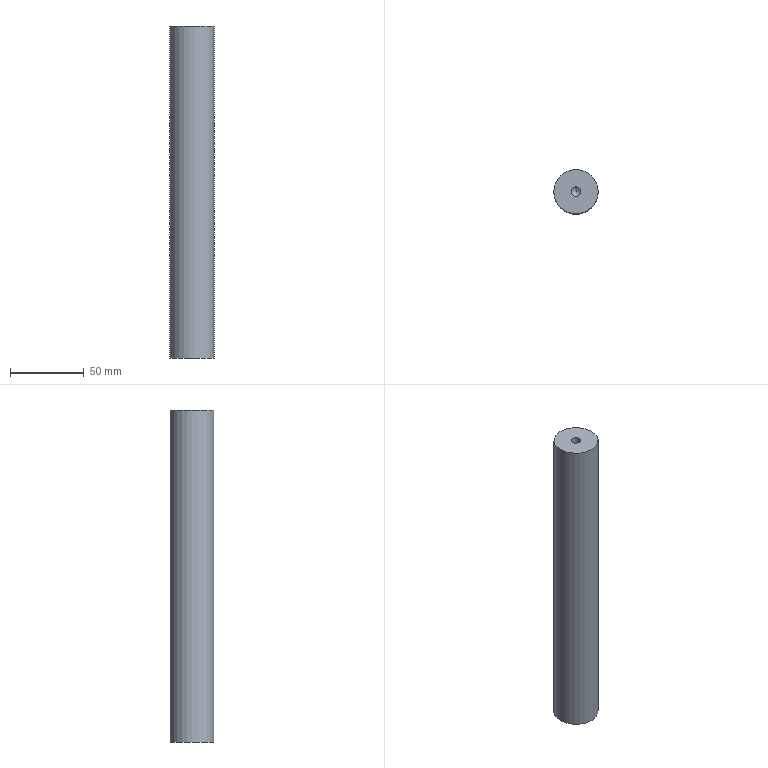Part | NX | features solid 2 | 1 solid | 7 faces | box 30 x 30 x 225 mm | volume 156454 mm3 | cylinder 3 | plane 2 | cone 2 | commonest cylinder face diameters 6.5 x1 8.782 x1 30 x1
STEP:
#1=CARTESIAN_POINT('',(-250.25,265.,-170.));
#2=VERTEX_POINT('',#1);
#3=CARTESIAN_POINT('',(-247.,265.,-170.));
#4=DIRECTION('',(0.,0.,-1.));
#5=DIRECTION('',(-1.,0.,0.));
#6=AXIS2_PLACEMENT_3D('',#3,#4,#5);
#7=CIRCLE('',#6,3.25);
#8=EDGE_CURVE('',#2,#2,#7,.T.);
#9=ORIENTED_EDGE('',*,*,#8,.T.);
#10=EDGE_LOOP('',(#9));
#11=FACE_BOUND('',#10,.T.);
#12=CARTESIAN_POINT('',(-232.,265.,-170.));
#13=VERTEX_POINT('',#12);
#14=CARTESIAN_POINT('',(-247.,265.,-170.));
#15=DIRECTION('',(0.,0.,1.));
#16=DIRECTION('',(1.,0.,0.));
#17=AXIS2_PLACEMENT_3D('',#14,#15,#16);
#18=CIRCLE('',#17,15.);
#19=EDGE_CURVE('',#13,#13,#18,.T.);
#20=ORIENTED_EDGE('',*,*,#19,.T.);
#21=EDGE_LOOP('',(#20));
#22=FACE_BOUND('',#21,.T.);
#23=CARTESIAN_POINT('',(-247.,285.,-170.));
#24=DIRECTION('',(0.,0.,-1.));
#25=DIRECTION('',(1.,0.,0.));
#26=AXIS2_PLACEMENT_3D('',#23,#24,#25);
#27=PLANE('',#26);
#28=ADVANCED_FACE('',(#11,#22),#27,.F.);
#29=CARTESIAN_POINT('',(-232.,265.,-395.));
#30=VERTEX_POINT('',#29);
#31=CARTESIAN_POINT('',(-247.,265.,-395.));
#32=DIRECTION('',(0.,0.,1.));
#33=DIRECTION('',(1.,0.,0.));
#34=AXIS2_PLACEMENT_3D('',#31,#32,#33);
#35=CIRCLE('',#34,15.);
#36=EDGE_CURVE('',#30,#30,#35,.T.);
#37=ORIENTED_EDGE('',*,*,#36,.T.);
#38=EDGE_LOOP('',(#37));
#39=FACE_BOUND('',#38,.T.);
#40=ORIENTED_EDGE('',*,*,#19,.F.);
#41=EDGE_LOOP('',(#40));
#42=FACE_BOUND('',#41,.T.);
#43=CARTESIAN_POINT('',(-247.,265.,-250.));
#44=DIRECTION('',(0.,0.,-1.));
#45=DIRECTION('',(1.,0.,0.));
#46=AXIS2_PLACEMENT_3D('',#43,#44,#45);
#47=CYLINDRICAL_SURFACE('',#46,15.);
#48=ADVANCED_FACE('',(#39,#42),#47,.T.);
#49=CARTESIAN_POINT('',(-242.609,265.,-395.));
#50=VERTEX_POINT('',#49);
#51=CARTESIAN_POINT('',(-247.,265.,-395.));
#52=DIRECTION('',(0.,0.,1.));
#53=DIRECTION('',(1.,0.,0.));
#54=AXIS2_PLACEMENT_3D('',#51,#52,#53);
#55=CIRCLE('',#54,4.391);
#56=EDGE_CURVE('',#50,#50,#55,.T.);
#57=ORIENTED_EDGE('',*,*,#56,.T.);
#58=EDGE_LOOP('',(#57));
#59=FACE_BOUND('',#58,.T.);
#60=ORIENTED_EDGE('',*,*,#36,.F.);
#61=EDGE_LOOP('',(#60));
#62=FACE_BOUND('',#61,.T.);
#63=CARTESIAN_POINT('',(-247.,265.,-395.));
#64=DIRECTION('',(0.,0.,-1.));
#65=DIRECTION('',(1.,0.,0.));
#66=AXIS2_PLACEMENT_3D('',#63,#64,#65);
#67=PLANE('',#66);
#68=ADVANCED_FACE('',(#59,#62),#67,.T.);
#69=CARTESIAN_POINT('',(-243.75,265.,-200.146));
#70=VERTEX_POINT('',#69);
#71=CARTESIAN_POINT('',(-247.,265.,-200.146));
#72=DIRECTION('',(0.,0.,1.));
#73=DIRECTION('',(1.,0.,0.));
#74=AXIS2_PLACEMENT_3D('',#71,#72,#73);
#75=CIRCLE('',#74,3.25);
#76=EDGE_CURVE('',#70,#70,#75,.F.);
#77=ORIENTED_EDGE('',*,*,#76,.F.);
#78=EDGE_LOOP('',(#77));
#79=FACE_BOUND('',#78,.T.);
#80=CARTESIAN_POINT('',(-247.,265.,-202.099));
#81=VERTEX_POINT('',#80);
#82=VERTEX_LOOP('',#81);
#83=FACE_BOUND('',#82,.T.);
#84=CARTESIAN_POINT('',(-247.,265.,-200.));
#85=DIRECTION('',(0.,0.,1.));
#86=DIRECTION('',(1.,0.,0.));
#87=AXIS2_PLACEMENT_3D('',#84,#85,#86);
#88=CONICAL_SURFACE('',#87,3.493,1.03);
#89=ADVANCED_FACE('',(#79,#83),#88,.F.);
#90=ORIENTED_EDGE('',*,*,#76,.T.);
#91=EDGE_LOOP('',(#90));
#92=FACE_BOUND('',#91,.T.);
#93=ORIENTED_EDGE('',*,*,#8,.F.);
#94=EDGE_LOOP('',(#93));
#95=FACE_BOUND('',#94,.T.);
#96=CARTESIAN_POINT('',(-247.,265.,-170.));
#97=DIRECTION('',(0.,0.,-1.));
#98=DIRECTION('',(-1.,0.,0.));
#99=AXIS2_PLACEMENT_3D('',#96,#97,#98);
#100=CYLINDRICAL_SURFACE('',#99,3.25);
#101=ADVANCED_FACE('',(#92,#95),#100,.F.);
#102=CARTESIAN_POINT('',(-242.609,265.,-370.));
#103=VERTEX_POINT('',#102);
#104=CARTESIAN_POINT('',(-247.,265.,-370.));
#105=DIRECTION('',(0.,0.,1.));
#106=DIRECTION('',(1.,0.,0.));
#107=AXIS2_PLACEMENT_3D('',#104,#105,#106);
#108=CIRCLE('',#107,4.391);
#109=EDGE_CURVE('',#103,#103,#108,.T.);
#110=ORIENTED_EDGE('',*,*,#109,.F.);
#111=EDGE_LOOP('',(#110));
#112=FACE_BOUND('',#111,.T.);
#113=CARTESIAN_POINT('',(-247.,265.,-367.362));
#114=VERTEX_POINT('',#113);
#115=VERTEX_LOOP('',#114);
#116=FACE_BOUND('',#115,.T.);
#117=CARTESIAN_POINT('',(-247.,265.,-370.));
#118=DIRECTION('',(0.,0.,-1.));
#119=DIRECTION('',(-1.,0.,0.));
#120=AXIS2_PLACEMENT_3D('',#117,#118,#119);
#121=CONICAL_SURFACE('',#120,4.391,1.03);
#122=ADVANCED_FACE('',(#112,#116),#121,.F.);
#123=ORIENTED_EDGE('',*,*,#109,.T.);
#124=EDGE_LOOP('',(#123));
#125=FACE_BOUND('',#124,.T.);
#126=ORIENTED_EDGE('',*,*,#56,.F.);
#127=EDGE_LOOP('',(#126));
#128=FACE_BOUND('',#127,.T.);
#129=CARTESIAN_POINT('',(-247.,265.,-395.));
#130=DIRECTION('',(0.,0.,1.));
#131=DIRECTION('',(1.,0.,0.));
#132=AXIS2_PLACEMENT_3D('',#129,#130,#131);
#133=CYLINDRICAL_SURFACE('',#132,4.391);
#134=ADVANCED_FACE('',(#125,#128),#133,.F.);
#135=CLOSED_SHELL('',(#28,#48,#68,#89,#101,#122,#134));
#136=MANIFOLD_SOLID_BREP('',#135);
#137=(LENGTH_UNIT()NAMED_UNIT(*)SI_UNIT(.MILLI.,.METRE.));
#138=UNCERTAINTY_MEASURE_WITH_UNIT(LENGTH_MEASURE(0.00001),#137,'','');
#139=(NAMED_UNIT(*)PLANE_ANGLE_UNIT()SI_UNIT($,.RADIAN.));
#140=(NAMED_UNIT(*)SI_UNIT($,.STERADIAN.)SOLID_ANGLE_UNIT());
#141=(GEOMETRIC_REPRESENTATION_CONTEXT(3)GLOBAL_UNCERTAINTY_ASSIGNED_CONTEXT((#138))GLOBAL_UNIT_ASSIGNED_CONTEXT((#137,#139,#140))REPRESENTATION_CONTEXT('',''));
#142=ADVANCED_BREP_SHAPE_REPRESENTATION('',(#136),#141);